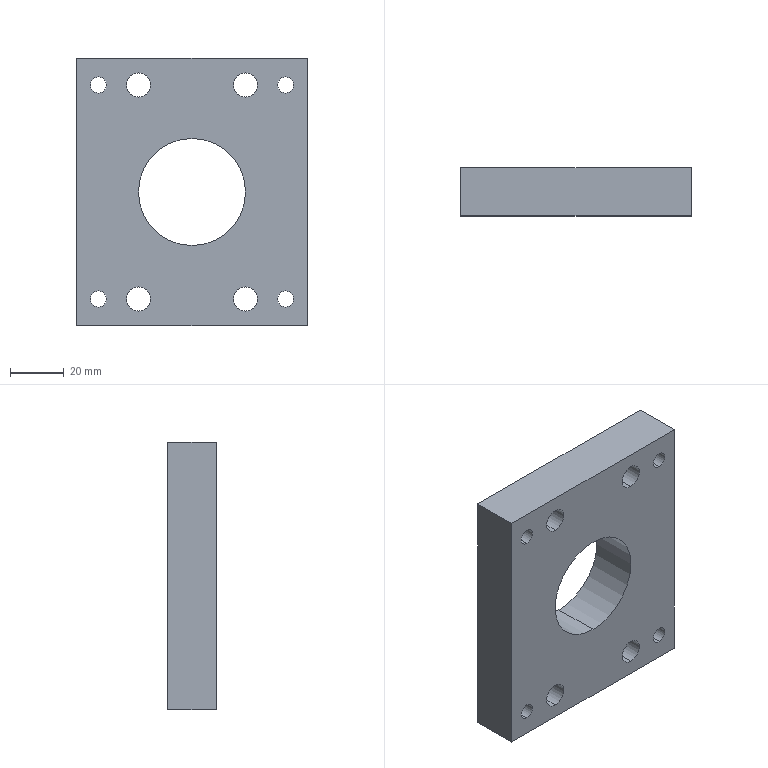Part | STEP file | 1 solid | 36 faces | box 86 x 18 x 100 mm | volume 121674 mm3 | cylinder 26 | plane 10 | commonest cylinder face diameters 6 x8 9 x8 15 x8 40 x2